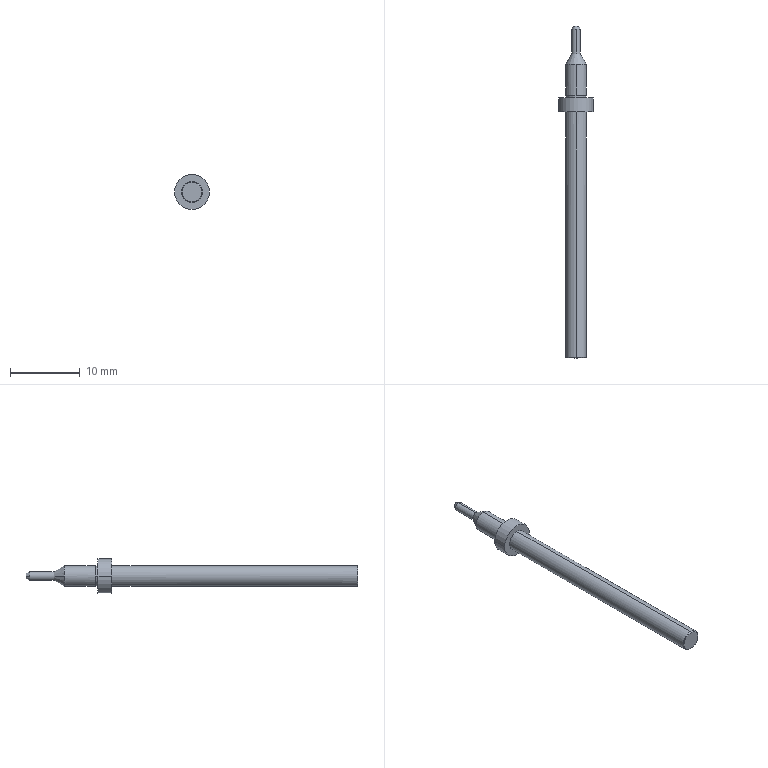Part | NX | 1 solid | 21 faces | box 5 x 47.5 x 5 mm | volume 332.204 mm3 | cylinder 10 | cone 6 | plane 5 | commonest cylinder face diameters 3 x4 1.28 x2 2.8 x2 5 x2
STEP:
#1=CARTESIAN_POINT('',(0.,25.2,-1.5));
#2=VERTEX_POINT('',#1);
#3=CARTESIAN_POINT('',(0.,25.2,1.5));
#4=VERTEX_POINT('',#3);
#5=CARTESIAN_POINT('',(0.,25.2,0.));
#6=DIRECTION('',(0.,-1.,0.));
#7=DIRECTION('',(0.,0.,1.));
#8=AXIS2_PLACEMENT_3D('',#5,#6,#7);
#9=CIRCLE('',#8,1.5);
#10=EDGE_CURVE('',#2,#4,#9,.T.);
#11=ORIENTED_EDGE('',*,*,#10,.T.);
#12=CARTESIAN_POINT('',(0.,-9.9,1.5));
#13=VERTEX_POINT('',#12);
#14=CARTESIAN_POINT('',(0.,39.875,1.5));
#15=DIRECTION('',(0.,-1.,0.));
#16=VECTOR('',#15,1000.);
#17=LINE('',#14,#16);
#18=EDGE_CURVE('',#4,#13,#17,.T.);
#19=ORIENTED_EDGE('',*,*,#18,.T.);
#20=CARTESIAN_POINT('',(1.5,-9.9,0.));
#21=VERTEX_POINT('',#20);
#22=CARTESIAN_POINT('',(0.,-9.9,0.));
#23=DIRECTION('',(0.,1.,0.));
#24=DIRECTION('',(1.,0.,0.));
#25=AXIS2_PLACEMENT_3D('',#22,#23,#24);
#26=CIRCLE('',#25,1.5);
#27=EDGE_CURVE('',#13,#21,#26,.T.);
#28=ORIENTED_EDGE('',*,*,#27,.T.);
#29=CARTESIAN_POINT('',(0.,-9.9,-1.5));
#30=VERTEX_POINT('',#29);
#31=CARTESIAN_POINT('',(0.,-9.9,0.));
#32=DIRECTION('',(0.,1.,0.));
#33=DIRECTION('',(1.,0.,0.));
#34=AXIS2_PLACEMENT_3D('',#31,#32,#33);
#35=CIRCLE('',#34,1.5);
#36=EDGE_CURVE('',#21,#30,#35,.T.);
#37=ORIENTED_EDGE('',*,*,#36,.T.);
#38=CARTESIAN_POINT('',(0.,39.875,-1.5));
#39=DIRECTION('',(0.,-1.,0.));
#40=VECTOR('',#39,1000.);
#41=LINE('',#38,#40);
#42=EDGE_CURVE('',#2,#30,#41,.T.);
#43=ORIENTED_EDGE('',*,*,#42,.F.);
#44=EDGE_LOOP('',(#11,#19,#28,#37,#43));
#45=FACE_BOUND('',#44,.T.);
#46=CARTESIAN_POINT('',(0.,39.875,0.));
#47=DIRECTION('',(0.,-1.,0.));
#48=DIRECTION('',(0.,0.,1.));
#49=AXIS2_PLACEMENT_3D('',#46,#47,#48);
#50=CYLINDRICAL_SURFACE('',#49,1.5);
#51=ADVANCED_FACE('',(#45),#50,.T.);
#52=CARTESIAN_POINT('',(-2.5,25.2,0.));
#53=VERTEX_POINT('',#52);
#54=CARTESIAN_POINT('',(2.5,25.2,0.));
#55=VERTEX_POINT('',#54);
#56=CARTESIAN_POINT('',(0.,25.2,0.));
#57=DIRECTION('',(0.,1.,0.));
#58=DIRECTION('',(1.,0.,0.));
#59=AXIS2_PLACEMENT_3D('',#56,#57,#58);
#60=CIRCLE('',#59,2.5);
#61=EDGE_CURVE('',#53,#55,#60,.T.);
#62=ORIENTED_EDGE('',*,*,#61,.F.);
#63=CARTESIAN_POINT('',(0.,25.2,0.));
#64=DIRECTION('',(0.,1.,0.));
#65=DIRECTION('',(1.,0.,0.));
#66=AXIS2_PLACEMENT_3D('',#63,#64,#65);
#67=CIRCLE('',#66,2.5);
#68=EDGE_CURVE('',#55,#53,#67,.T.);
#69=ORIENTED_EDGE('',*,*,#68,.F.);
#70=EDGE_LOOP('',(#62,#69));
#71=FACE_BOUND('',#70,.T.);
#72=ORIENTED_EDGE('',*,*,#10,.F.);
#73=CARTESIAN_POINT('',(0.,25.2,0.));
#74=DIRECTION('',(0.,-1.,0.));
#75=DIRECTION('',(0.,0.,1.));
#76=AXIS2_PLACEMENT_3D('',#73,#74,#75);
#77=CIRCLE('',#76,1.5);
#78=EDGE_CURVE('',#4,#2,#77,.T.);
#79=ORIENTED_EDGE('',*,*,#78,.F.);
#80=EDGE_LOOP('',(#72,#79));
#81=FACE_BOUND('',#80,.T.);
#82=CARTESIAN_POINT('',(0.,25.2,0.));
#83=DIRECTION('',(0.,-1.,0.));
#84=DIRECTION('',(0.,0.,-1.));
#85=AXIS2_PLACEMENT_3D('',#82,#83,#84);
#86=PLANE('',#85);
#87=ADVANCED_FACE('',(#71,#81),#86,.T.);
#88=CARTESIAN_POINT('',(2.5,27.2,0.));
#89=VERTEX_POINT('',#88);
#90=CARTESIAN_POINT('',(-2.5,27.2,0.));
#91=VERTEX_POINT('',#90);
#92=CARTESIAN_POINT('',(0.,27.2,0.));
#93=DIRECTION('',(0.,-1.,0.));
#94=DIRECTION('',(-1.,0.,0.));
#95=AXIS2_PLACEMENT_3D('',#92,#93,#94);
#96=CIRCLE('',#95,2.5);
#97=EDGE_CURVE('',#89,#91,#96,.T.);
#98=ORIENTED_EDGE('',*,*,#97,.T.);
#99=CARTESIAN_POINT('',(-2.5,27.2,0.));
#100=DIRECTION('',(0.,-1.,0.));
#101=VECTOR('',#100,1000.);
#102=LINE('',#99,#101);
#103=EDGE_CURVE('',#91,#53,#102,.T.);
#104=ORIENTED_EDGE('',*,*,#103,.T.);
#105=ORIENTED_EDGE('',*,*,#61,.T.);
#106=CARTESIAN_POINT('',(2.5,27.2,0.));
#107=DIRECTION('',(0.,-1.,0.));
#108=VECTOR('',#107,1000.);
#109=LINE('',#106,#108);
#110=EDGE_CURVE('',#89,#55,#109,.T.);
#111=ORIENTED_EDGE('',*,*,#110,.F.);
#112=EDGE_LOOP('',(#98,#104,#105,#111));
#113=FACE_BOUND('',#112,.T.);
#114=CARTESIAN_POINT('',(0.,27.2,0.));
#115=DIRECTION('',(0.,-1.,0.));
#116=DIRECTION('',(1.,0.,0.));
#117=AXIS2_PLACEMENT_3D('',#114,#115,#116);
#118=CYLINDRICAL_SURFACE('',#117,2.5);
#119=ADVANCED_FACE('',(#113),#118,.T.);
#120=CARTESIAN_POINT('',(0.,27.6,1.5));
#121=VERTEX_POINT('',#120);
#122=CARTESIAN_POINT('',(0.,27.6,-1.5));
#123=VERTEX_POINT('',#122);
#124=CARTESIAN_POINT('',(0.,27.6,0.));
#125=DIRECTION('',(0.,-1.,0.));
#126=DIRECTION('',(0.,0.,1.));
#127=AXIS2_PLACEMENT_3D('',#124,#125,#126);
#128=CIRCLE('',#127,1.5);
#129=EDGE_CURVE('',#121,#123,#128,.T.);
#130=ORIENTED_EDGE('',*,*,#129,.T.);
#131=CARTESIAN_POINT('',(0.,27.6,0.));
#132=DIRECTION('',(0.,-1.,0.));
#133=DIRECTION('',(0.,0.,1.));
#134=AXIS2_PLACEMENT_3D('',#131,#132,#133);
#135=CIRCLE('',#134,1.5);
#136=EDGE_CURVE('',#123,#121,#135,.T.);
#137=ORIENTED_EDGE('',*,*,#136,.T.);
#138=EDGE_LOOP('',(#130,#137));
#139=FACE_BOUND('',#138,.T.);
#140=CARTESIAN_POINT('',(1.4,27.6,0.));
#141=VERTEX_POINT('',#140);
#142=CARTESIAN_POINT('',(-1.4,27.6,0.));
#143=VERTEX_POINT('',#142);
#144=CARTESIAN_POINT('',(0.,27.6,0.));
#145=DIRECTION('',(0.,1.,0.));
#146=DIRECTION('',(1.,0.,0.));
#147=AXIS2_PLACEMENT_3D('',#144,#145,#146);
#148=CIRCLE('',#147,1.4);
#149=EDGE_CURVE('',#141,#143,#148,.T.);
#150=ORIENTED_EDGE('',*,*,#149,.T.);
#151=CARTESIAN_POINT('',(0.,27.6,0.));
#152=DIRECTION('',(0.,1.,0.));
#153=DIRECTION('',(1.,0.,0.));
#154=AXIS2_PLACEMENT_3D('',#151,#152,#153);
#155=CIRCLE('',#154,1.4);
#156=EDGE_CURVE('',#143,#141,#155,.T.);
#157=ORIENTED_EDGE('',*,*,#156,.T.);
#158=EDGE_LOOP('',(#150,#157));
#159=FACE_BOUND('',#158,.T.);
#160=CARTESIAN_POINT('',(0.,27.6,0.));
#161=DIRECTION('',(0.,1.,0.));
#162=DIRECTION('',(1.,0.,0.));
#163=AXIS2_PLACEMENT_3D('',#160,#161,#162);
#164=PLANE('',#163);
#165=ADVANCED_FACE('',(#139,#159),#164,.F.);
#166=CARTESIAN_POINT('',(-1.4,-10.,0.));
#167=VERTEX_POINT('',#166);
#168=CARTESIAN_POINT('',(1.4,-10.,0.));
#169=VERTEX_POINT('',#168);
#170=CARTESIAN_POINT('',(0.,-10.,0.));
#171=DIRECTION('',(0.,1.,0.));
#172=DIRECTION('',(1.,0.,0.));
#173=AXIS2_PLACEMENT_3D('',#170,#171,#172);
#174=CIRCLE('',#173,1.4);
#175=EDGE_CURVE('',#167,#169,#174,.T.);
#176=ORIENTED_EDGE('',*,*,#175,.F.);
#177=CARTESIAN_POINT('',(0.,-10.,0.));
#178=DIRECTION('',(0.,1.,0.));
#179=DIRECTION('',(1.,0.,0.));
#180=AXIS2_PLACEMENT_3D('',#177,#178,#179);
#181=CIRCLE('',#180,1.4);
#182=EDGE_CURVE('',#169,#167,#181,.T.);
#183=ORIENTED_EDGE('',*,*,#182,.F.);
#184=EDGE_LOOP('',(#176,#183));
#185=FACE_BOUND('',#184,.T.);
#186=CARTESIAN_POINT('',(0.,-10.,0.));
#187=DIRECTION('',(0.,-1.,0.));
#188=DIRECTION('',(0.,0.,-1.));
#189=AXIS2_PLACEMENT_3D('',#186,#187,#188);
#190=PLANE('',#189);
#191=ADVANCED_FACE('',(#185),#190,.T.);
#192=CARTESIAN_POINT('',(1.4,27.2,0.));
#193=VERTEX_POINT('',#192);
#194=CARTESIAN_POINT('',(-1.4,27.2,0.));
#195=VERTEX_POINT('',#194);
#196=CARTESIAN_POINT('',(0.,27.2,0.));
#197=DIRECTION('',(0.,1.,0.));
#198=DIRECTION('',(1.,0.,0.));
#199=AXIS2_PLACEMENT_3D('',#196,#197,#198);
#200=CIRCLE('',#199,1.4);
#201=EDGE_CURVE('',#193,#195,#200,.T.);
#202=ORIENTED_EDGE('',*,*,#201,.T.);
#203=CARTESIAN_POINT('',(-1.4,27.195,0.));
#204=DIRECTION('',(0.,1.,0.));
#205=VECTOR('',#204,1000.);
#206=LINE('',#203,#205);
#207=EDGE_CURVE('',#195,#143,#206,.T.);
#208=ORIENTED_EDGE('',*,*,#207,.T.);
#209=ORIENTED_EDGE('',*,*,#149,.F.);
#210=CARTESIAN_POINT('',(1.4,27.195,0.));
#211=DIRECTION('',(0.,1.,0.));
#212=VECTOR('',#211,1000.);
#213=LINE('',#210,#212);
#214=EDGE_CURVE('',#193,#141,#213,.T.);
#215=ORIENTED_EDGE('',*,*,#214,.F.);
#216=EDGE_LOOP('',(#202,#208,#209,#215));
#217=FACE_BOUND('',#216,.T.);
#218=CARTESIAN_POINT('',(0.,27.195,0.));
#219=DIRECTION('',(0.,1.,0.));
#220=DIRECTION('',(1.,0.,0.));
#221=AXIS2_PLACEMENT_3D('',#218,#219,#220);
#222=CYLINDRICAL_SURFACE('',#221,1.4);
#223=ADVANCED_FACE('',(#217),#222,.T.);
#224=CARTESIAN_POINT('',(0.4068,37.5,0.));
#225=VERTEX_POINT('',#224);
#226=CARTESIAN_POINT('',(-0.4068,37.5,0.));
#227=VERTEX_POINT('',#226);
#228=CARTESIAN_POINT('',(0.,37.5,0.));
#229=DIRECTION('',(0.,-1.,0.));
#230=DIRECTION('',(-1.,0.,0.));
#231=AXIS2_PLACEMENT_3D('',#228,#229,#230);
#232=CIRCLE('',#231,0.4068);
#233=EDGE_CURVE('',#225,#227,#232,.T.);
#234=ORIENTED_EDGE('',*,*,#233,.F.);
#235=CARTESIAN_POINT('',(0.,37.5,0.));
#236=DIRECTION('',(0.,-1.,0.));
#237=DIRECTION('',(-1.,0.,0.));
#238=AXIS2_PLACEMENT_3D('',#235,#236,#237);
#239=CIRCLE('',#238,0.4068);
#240=EDGE_CURVE('',#227,#225,#239,.T.);
#241=ORIENTED_EDGE('',*,*,#240,.F.);
#242=EDGE_LOOP('',(#234,#241));
#243=FACE_BOUND('',#242,.T.);
#244=CARTESIAN_POINT('',(0.,37.5,0.));
#245=DIRECTION('',(0.,-1.,0.));
#246=DIRECTION('',(0.,0.,-1.));
#247=AXIS2_PLACEMENT_3D('',#244,#245,#246);
#248=PLANE('',#247);
#249=ADVANCED_FACE('',(#243),#248,.F.);
#250=ORIENTED_EDGE('',*,*,#97,.F.);
#251=CARTESIAN_POINT('',(0.,27.2,0.));
#252=DIRECTION('',(0.,-1.,0.));
#253=DIRECTION('',(-1.,0.,0.));
#254=AXIS2_PLACEMENT_3D('',#251,#252,#253);
#255=CIRCLE('',#254,2.5);
#256=EDGE_CURVE('',#91,#89,#255,.T.);
#257=ORIENTED_EDGE('',*,*,#256,.F.);
#258=EDGE_LOOP('',(#250,#257));
#259=FACE_BOUND('',#258,.T.);
#260=ORIENTED_EDGE('',*,*,#201,.F.);
#261=CARTESIAN_POINT('',(0.,27.2,0.));
#262=DIRECTION('',(0.,1.,0.));
#263=DIRECTION('',(1.,0.,0.));
#264=AXIS2_PLACEMENT_3D('',#261,#262,#263);
#265=CIRCLE('',#264,1.4);
#266=EDGE_CURVE('',#195,#193,#265,.T.);
#267=ORIENTED_EDGE('',*,*,#266,.F.);
#268=EDGE_LOOP('',(#260,#267));
#269=FACE_BOUND('',#268,.T.);
#270=CARTESIAN_POINT('',(0.,27.2,0.));
#271=DIRECTION('',(0.,-1.,0.));
#272=DIRECTION('',(0.,0.,-1.));
#273=AXIS2_PLACEMENT_3D('',#270,#271,#272);
#274=PLANE('',#273);
#275=ADVANCED_FACE('',(#259,#269),#274,.F.);
#276=CARTESIAN_POINT('',(-1.5,32.,0.));
#277=VERTEX_POINT('',#276);
#278=CARTESIAN_POINT('',(0.,32.,-1.5));
#279=VERTEX_POINT('',#278);
#280=CARTESIAN_POINT('',(0.,32.,0.));
#281=DIRECTION('',(0.,-1.,0.));
#282=DIRECTION('',(-1.,0.,0.));
#283=AXIS2_PLACEMENT_3D('',#280,#281,#282);
#284=CIRCLE('',#283,1.5);
#285=EDGE_CURVE('',#277,#279,#284,.T.);
#286=ORIENTED_EDGE('',*,*,#285,.T.);
#287=CARTESIAN_POINT('',(0.,39.875,-1.5));
#288=DIRECTION('',(0.,-1.,0.));
#289=VECTOR('',#288,1000.);
#290=LINE('',#287,#289);
#291=EDGE_CURVE('',#279,#123,#290,.T.);
#292=ORIENTED_EDGE('',*,*,#291,.T.);
#293=ORIENTED_EDGE('',*,*,#129,.F.);
#294=CARTESIAN_POINT('',(0.,32.,1.5));
#295=VERTEX_POINT('',#294);
#296=CARTESIAN_POINT('',(0.,39.875,1.5));
#297=DIRECTION('',(0.,-1.,0.));
#298=VECTOR('',#297,1000.);
#299=LINE('',#296,#298);
#300=EDGE_CURVE('',#295,#121,#299,.T.);
#301=ORIENTED_EDGE('',*,*,#300,.F.);
#302=CARTESIAN_POINT('',(0.,32.,0.));
#303=DIRECTION('',(0.,-1.,0.));
#304=DIRECTION('',(-1.,0.,0.));
#305=AXIS2_PLACEMENT_3D('',#302,#303,#304);
#306=CIRCLE('',#305,1.5);
#307=EDGE_CURVE('',#295,#277,#306,.T.);
#308=ORIENTED_EDGE('',*,*,#307,.T.);
#309=EDGE_LOOP('',(#286,#292,#293,#301,#308));
#310=FACE_BOUND('',#309,.T.);
#311=CARTESIAN_POINT('',(0.,39.875,0.));
#312=DIRECTION('',(0.,-1.,0.));
#313=DIRECTION('',(0.,0.,1.));
#314=AXIS2_PLACEMENT_3D('',#311,#312,#313);
#315=CYLINDRICAL_SURFACE('',#314,1.5);
#316=ADVANCED_FACE('',(#310),#315,.T.);
#317=CARTESIAN_POINT('',(0.,37.,0.64));
#318=VERTEX_POINT('',#317);
#319=CARTESIAN_POINT('',(-0.64,37.,0.));
#320=VERTEX_POINT('',#319);
#321=CARTESIAN_POINT('',(0.,37.,0.));
#322=DIRECTION('',(0.,-1.,0.));
#323=DIRECTION('',(-1.,0.,0.));
#324=AXIS2_PLACEMENT_3D('',#321,#322,#323);
#325=CIRCLE('',#324,0.64);
#326=EDGE_CURVE('',#318,#320,#325,.T.);
#327=ORIENTED_EDGE('',*,*,#326,.T.);
#328=CARTESIAN_POINT('',(0.,37.,-0.64));
#329=VERTEX_POINT('',#328);
#330=CARTESIAN_POINT('',(0.,37.,0.));
#331=DIRECTION('',(0.,-1.,0.));
#332=DIRECTION('',(-1.,0.,0.));
#333=AXIS2_PLACEMENT_3D('',#330,#331,#332);
#334=CIRCLE('',#333,0.64);
#335=EDGE_CURVE('',#320,#329,#334,.T.);
#336=ORIENTED_EDGE('',*,*,#335,.T.);
#337=CARTESIAN_POINT('',(0.,33.49,-0.64));
#338=VERTEX_POINT('',#337);
#339=CARTESIAN_POINT('',(0.,39.875,-0.64));
#340=DIRECTION('',(0.,-1.,0.));
#341=VECTOR('',#340,1000.);
#342=LINE('',#339,#341);
#343=EDGE_CURVE('',#338,#329,#342,.F.);
#344=ORIENTED_EDGE('',*,*,#343,.F.);
#345=CARTESIAN_POINT('',(-0.64,33.49,0.));
#346=VERTEX_POINT('',#345);
#347=CARTESIAN_POINT('',(0.,33.49,0.));
#348=DIRECTION('',(0.,-1.,0.));
#349=DIRECTION('',(-1.,0.,0.));
#350=AXIS2_PLACEMENT_3D('',#347,#348,#349);
#351=CIRCLE('',#350,0.64);
#352=EDGE_CURVE('',#346,#338,#351,.T.);
#353=ORIENTED_EDGE('',*,*,#352,.F.);
#354=CARTESIAN_POINT('',(0.,33.49,0.64));
#355=VERTEX_POINT('',#354);
#356=CARTESIAN_POINT('',(0.,33.49,0.));
#357=DIRECTION('',(0.,-1.,0.));
#358=DIRECTION('',(-1.,0.,0.));
#359=AXIS2_PLACEMENT_3D('',#356,#357,#358);
#360=CIRCLE('',#359,0.64);
#361=EDGE_CURVE('',#355,#346,#360,.T.);
#362=ORIENTED_EDGE('',*,*,#361,.F.);
#363=CARTESIAN_POINT('',(0.,39.875,0.64));
#364=DIRECTION('',(0.,-1.,0.));
#365=VECTOR('',#364,1000.);
#366=LINE('',#363,#365);
#367=EDGE_CURVE('',#355,#318,#366,.F.);
#368=ORIENTED_EDGE('',*,*,#367,.T.);
#369=EDGE_LOOP('',(#327,#336,#344,#353,#362,#368));
#370=FACE_BOUND('',#369,.T.);
#371=CARTESIAN_POINT('',(0.,39.875,0.));
#372=DIRECTION('',(0.,-1.,0.));
#373=DIRECTION('',(0.,0.,1.));
#374=AXIS2_PLACEMENT_3D('',#371,#372,#373);
#375=CYLINDRICAL_SURFACE('',#374,0.64);
#376=ADVANCED_FACE('',(#370),#375,.T.);
#377=ORIENTED_EDGE('',*,*,#285,.F.);
#378=CARTESIAN_POINT('',(-1.07,32.745,0.));
#379=DIRECTION('',(-0.5,-0.866,0.));
#380=VECTOR('',#379,1000.);
#381=LINE('',#378,#380);
#382=EDGE_CURVE('',#277,#346,#381,.F.);
#383=ORIENTED_EDGE('',*,*,#382,.T.);
#384=ORIENTED_EDGE('',*,*,#352,.T.);
#385=CARTESIAN_POINT('',(0.64,33.49,0.));
#386=VERTEX_POINT('',#385);
#387=CARTESIAN_POINT('',(0.,33.49,0.));
#388=DIRECTION('',(0.,-1.,0.));
#389=DIRECTION('',(-1.,0.,0.));
#390=AXIS2_PLACEMENT_3D('',#387,#388,#389);
#391=CIRCLE('',#390,0.64);
#392=EDGE_CURVE('',#338,#386,#391,.T.);
#393=ORIENTED_EDGE('',*,*,#392,.T.);
#394=CARTESIAN_POINT('',(1.5,32.,0.));
#395=VERTEX_POINT('',#394);
#396=CARTESIAN_POINT('',(1.07,32.745,0.));
#397=DIRECTION('',(0.5,-0.866,0.));
#398=VECTOR('',#397,1000.);
#399=LINE('',#396,#398);
#400=EDGE_CURVE('',#395,#386,#399,.F.);
#401=ORIENTED_EDGE('',*,*,#400,.F.);
#402=CARTESIAN_POINT('',(0.,32.,0.));
#403=DIRECTION('',(0.,-1.,0.));
#404=DIRECTION('',(-1.,0.,0.));
#405=AXIS2_PLACEMENT_3D('',#402,#403,#404);
#406=CIRCLE('',#405,1.5);
#407=EDGE_CURVE('',#279,#395,#406,.T.);
#408=ORIENTED_EDGE('',*,*,#407,.F.);
#409=EDGE_LOOP('',(#377,#383,#384,#393,#401,#408));
#410=FACE_BOUND('',#409,.T.);
#411=CARTESIAN_POINT('',(0.,32.745,0.));
#412=DIRECTION('',(0.,-1.,0.));
#413=DIRECTION('',(-1.,0.,0.));
#414=AXIS2_PLACEMENT_3D('',#411,#412,#413);
#415=CONICAL_SURFACE('',#414,1.07,0.5236);
#416=ADVANCED_FACE('',(#410),#415,.T.);
#417=ORIENTED_EDGE('',*,*,#326,.F.);
#418=CARTESIAN_POINT('',(0.64,37.,0.));
#419=VERTEX_POINT('',#418);
#420=CARTESIAN_POINT('',(0.,37.,0.));
#421=DIRECTION('',(0.,-1.,0.));
#422=DIRECTION('',(-1.,0.,0.));
#423=AXIS2_PLACEMENT_3D('',#420,#421,#422);
#424=CIRCLE('',#423,0.64);
#425=EDGE_CURVE('',#419,#318,#424,.T.);
#426=ORIENTED_EDGE('',*,*,#425,.F.);
#427=CARTESIAN_POINT('',(0.64,37.,0.));
#428=DIRECTION('',(0.4226,-0.9063,0.));
#429=VECTOR('',#428,1000.);
#430=LINE('',#427,#429);
#431=EDGE_CURVE('',#419,#225,#430,.F.);
#432=ORIENTED_EDGE('',*,*,#431,.T.);
#433=ORIENTED_EDGE('',*,*,#233,.T.);
#434=CARTESIAN_POINT('',(-0.64,37.,0.));
#435=DIRECTION('',(-0.4226,-0.9063,0.));
#436=VECTOR('',#435,1000.);
#437=LINE('',#434,#436);
#438=EDGE_CURVE('',#320,#227,#437,.F.);
#439=ORIENTED_EDGE('',*,*,#438,.F.);
#440=EDGE_LOOP('',(#417,#426,#432,#433,#439));
#441=FACE_BOUND('',#440,.T.);
#442=CARTESIAN_POINT('',(0.,37.,0.));
#443=DIRECTION('',(0.,-1.,0.));
#444=DIRECTION('',(-1.,0.,0.));
#445=AXIS2_PLACEMENT_3D('',#442,#443,#444);
#446=CONICAL_SURFACE('',#445,0.64,0.4363);
#447=ADVANCED_FACE('',(#441),#446,.T.);
#448=ORIENTED_EDGE('',*,*,#175,.T.);
#449=CARTESIAN_POINT('',(1.5,-9.9,0.));
#450=DIRECTION('',(0.7071,0.7071,0.));
#451=VECTOR('',#450,1000.);
#452=LINE('',#449,#451);
#453=EDGE_CURVE('',#169,#21,#452,.T.);
#454=ORIENTED_EDGE('',*,*,#453,.T.);
#455=ORIENTED_EDGE('',*,*,#27,.F.);
#456=CARTESIAN_POINT('',(-1.5,-9.9,0.));
#457=VERTEX_POINT('',#456);
#458=CARTESIAN_POINT('',(0.,-9.9,0.));
#459=DIRECTION('',(0.,1.,0.));
#460=DIRECTION('',(1.,0.,0.));
#461=AXIS2_PLACEMENT_3D('',#458,#459,#460);
#462=CIRCLE('',#461,1.5);
#463=EDGE_CURVE('',#457,#13,#462,.T.);
#464=ORIENTED_EDGE('',*,*,#463,.F.);
#465=CARTESIAN_POINT('',(-1.5,-9.9,0.));
#466=DIRECTION('',(-0.7071,0.7071,0.));
#467=VECTOR('',#466,1000.);
#468=LINE('',#465,#467);
#469=EDGE_CURVE('',#167,#457,#468,.T.);
#470=ORIENTED_EDGE('',*,*,#469,.F.);
#471=EDGE_LOOP('',(#448,#454,#455,#464,#470));
#472=FACE_BOUND('',#471,.T.);
#473=CARTESIAN_POINT('',(0.,-9.9,0.));
#474=DIRECTION('',(0.,1.,0.));
#475=DIRECTION('',(1.,0.,0.));
#476=AXIS2_PLACEMENT_3D('',#473,#474,#475);
#477=CONICAL_SURFACE('',#476,1.5,0.7854);
#478=ADVANCED_FACE('',(#472),#477,.T.);
#479=ORIENTED_EDGE('',*,*,#382,.F.);
#480=ORIENTED_EDGE('',*,*,#307,.F.);
#481=CARTESIAN_POINT('',(0.,32.,0.));
#482=DIRECTION('',(0.,-1.,0.));
#483=DIRECTION('',(-1.,0.,0.));
#484=AXIS2_PLACEMENT_3D('',#481,#482,#483);
#485=CIRCLE('',#484,1.5);
#486=EDGE_CURVE('',#395,#295,#485,.T.);
#487=ORIENTED_EDGE('',*,*,#486,.F.);
#488=ORIENTED_EDGE('',*,*,#400,.T.);
#489=CARTESIAN_POINT('',(0.,33.49,0.));
#490=DIRECTION('',(0.,-1.,0.));
#491=DIRECTION('',(-1.,0.,0.));
#492=AXIS2_PLACEMENT_3D('',#489,#490,#491);
#493=CIRCLE('',#492,0.64);
#494=EDGE_CURVE('',#386,#355,#493,.T.);
#495=ORIENTED_EDGE('',*,*,#494,.T.);
#496=ORIENTED_EDGE('',*,*,#361,.T.);
#497=EDGE_LOOP('',(#479,#480,#487,#488,#495,#496));
#498=FACE_BOUND('',#497,.T.);
#499=CARTESIAN_POINT('',(0.,32.745,0.));
#500=DIRECTION('',(0.,-1.,0.));
#501=DIRECTION('',(-1.,0.,0.));
#502=AXIS2_PLACEMENT_3D('',#499,#500,#501);
#503=CONICAL_SURFACE('',#502,1.07,0.5236);
#504=ADVANCED_FACE('',(#498),#503,.T.);
#505=ORIENTED_EDGE('',*,*,#214,.T.);
#506=ORIENTED_EDGE('',*,*,#156,.F.);
#507=ORIENTED_EDGE('',*,*,#207,.F.);
#508=ORIENTED_EDGE('',*,*,#266,.T.);
#509=EDGE_LOOP('',(#505,#506,#507,#508));
#510=FACE_BOUND('',#509,.T.);
#511=CARTESIAN_POINT('',(0.,27.195,0.));
#512=DIRECTION('',(0.,1.,0.));
#513=DIRECTION('',(1.,0.,0.));
#514=AXIS2_PLACEMENT_3D('',#511,#512,#513);
#515=CYLINDRICAL_SURFACE('',#514,1.4);
#516=ADVANCED_FACE('',(#510),#515,.T.);
#517=ORIENTED_EDGE('',*,*,#453,.F.);
#518=ORIENTED_EDGE('',*,*,#182,.T.);
#519=ORIENTED_EDGE('',*,*,#469,.T.);
#520=CARTESIAN_POINT('',(0.,-9.9,0.));
#521=DIRECTION('',(0.,1.,0.));
#522=DIRECTION('',(1.,0.,0.));
#523=AXIS2_PLACEMENT_3D('',#520,#521,#522);
#524=CIRCLE('',#523,1.5);
#525=EDGE_CURVE('',#30,#457,#524,.T.);
#526=ORIENTED_EDGE('',*,*,#525,.F.);
#527=ORIENTED_EDGE('',*,*,#36,.F.);
#528=EDGE_LOOP('',(#517,#518,#519,#526,#527));
#529=FACE_BOUND('',#528,.T.);
#530=CARTESIAN_POINT('',(0.,-9.9,0.));
#531=DIRECTION('',(0.,1.,0.));
#532=DIRECTION('',(1.,0.,0.));
#533=AXIS2_PLACEMENT_3D('',#530,#531,#532);
#534=CONICAL_SURFACE('',#533,1.5,0.7854);
#535=ADVANCED_FACE('',(#529),#534,.T.);
#536=ORIENTED_EDGE('',*,*,#392,.F.);
#537=ORIENTED_EDGE('',*,*,#343,.T.);
#538=CARTESIAN_POINT('',(0.,37.,0.));
#539=DIRECTION('',(0.,-1.,0.));
#540=DIRECTION('',(-1.,0.,0.));
#541=AXIS2_PLACEMENT_3D('',#538,#539,#540);
#542=CIRCLE('',#541,0.64);
#543=EDGE_CURVE('',#329,#419,#542,.T.);
#544=ORIENTED_EDGE('',*,*,#543,.T.);
#545=ORIENTED_EDGE('',*,*,#425,.T.);
#546=ORIENTED_EDGE('',*,*,#367,.F.);
#547=ORIENTED_EDGE('',*,*,#494,.F.);
#548=EDGE_LOOP('',(#536,#537,#544,#545,#546,#547));
#549=FACE_BOUND('',#548,.T.);
#550=CARTESIAN_POINT('',(0.,39.875,0.));
#551=DIRECTION('',(0.,-1.,0.));
#552=DIRECTION('',(0.,0.,1.));
#553=AXIS2_PLACEMENT_3D('',#550,#551,#552);
#554=CYLINDRICAL_SURFACE('',#553,0.64);
#555=ADVANCED_FACE('',(#549),#554,.T.);
#556=ORIENTED_EDGE('',*,*,#110,.T.);
#557=ORIENTED_EDGE('',*,*,#68,.T.);
#558=ORIENTED_EDGE('',*,*,#103,.F.);
#559=ORIENTED_EDGE('',*,*,#256,.T.);
#560=EDGE_LOOP('',(#556,#557,#558,#559));
#561=FACE_BOUND('',#560,.T.);
#562=CARTESIAN_POINT('',(0.,27.2,0.));
#563=DIRECTION('',(0.,-1.,0.));
#564=DIRECTION('',(1.,0.,0.));
#565=AXIS2_PLACEMENT_3D('',#562,#563,#564);
#566=CYLINDRICAL_SURFACE('',#565,2.5);
#567=ADVANCED_FACE('',(#561),#566,.T.);
#568=ORIENTED_EDGE('',*,*,#438,.T.);
#569=ORIENTED_EDGE('',*,*,#240,.T.);
#570=ORIENTED_EDGE('',*,*,#431,.F.);
#571=ORIENTED_EDGE('',*,*,#543,.F.);
#572=ORIENTED_EDGE('',*,*,#335,.F.);
#573=EDGE_LOOP('',(#568,#569,#570,#571,#572));
#574=FACE_BOUND('',#573,.T.);
#575=CARTESIAN_POINT('',(0.,37.,0.));
#576=DIRECTION('',(0.,-1.,0.));
#577=DIRECTION('',(-1.,0.,0.));
#578=AXIS2_PLACEMENT_3D('',#575,#576,#577);
#579=CONICAL_SURFACE('',#578,0.64,0.4363);
#580=ADVANCED_FACE('',(#574),#579,.T.);
#581=ORIENTED_EDGE('',*,*,#300,.T.);
#582=ORIENTED_EDGE('',*,*,#136,.F.);
#583=ORIENTED_EDGE('',*,*,#291,.F.);
#584=ORIENTED_EDGE('',*,*,#407,.T.);
#585=ORIENTED_EDGE('',*,*,#486,.T.);
#586=EDGE_LOOP('',(#581,#582,#583,#584,#585));
#587=FACE_BOUND('',#586,.T.);
#588=CARTESIAN_POINT('',(0.,39.875,0.));
#589=DIRECTION('',(0.,-1.,0.));
#590=DIRECTION('',(0.,0.,1.));
#591=AXIS2_PLACEMENT_3D('',#588,#589,#590);
#592=CYLINDRICAL_SURFACE('',#591,1.5);
#593=ADVANCED_FACE('',(#587),#592,.T.);
#594=ORIENTED_EDGE('',*,*,#463,.T.);
#595=ORIENTED_EDGE('',*,*,#18,.F.);
#596=ORIENTED_EDGE('',*,*,#78,.T.);
#597=ORIENTED_EDGE('',*,*,#42,.T.);
#598=ORIENTED_EDGE('',*,*,#525,.T.);
#599=EDGE_LOOP('',(#594,#595,#596,#597,#598));
#600=FACE_BOUND('',#599,.T.);
#601=CARTESIAN_POINT('',(0.,39.875,0.));
#602=DIRECTION('',(0.,-1.,0.));
#603=DIRECTION('',(0.,0.,1.));
#604=AXIS2_PLACEMENT_3D('',#601,#602,#603);
#605=CYLINDRICAL_SURFACE('',#604,1.5);
#606=ADVANCED_FACE('',(#600),#605,.T.);
#607=CLOSED_SHELL('',(#51,#87,#119,#165,#191,#223,#249,#275,#316,#376,#416,#447,#478,#504,#516,#535,#555,#567,#580,#593,#606));
#608=MANIFOLD_SOLID_BREP('',#607);
#609=(LENGTH_UNIT()NAMED_UNIT(*)SI_UNIT(.MILLI.,.METRE.));
#610=UNCERTAINTY_MEASURE_WITH_UNIT(LENGTH_MEASURE(0.00001),#609,'','');
#611=(NAMED_UNIT(*)PLANE_ANGLE_UNIT()SI_UNIT($,.RADIAN.));
#612=(NAMED_UNIT(*)SI_UNIT($,.STERADIAN.)SOLID_ANGLE_UNIT());
#613=(GEOMETRIC_REPRESENTATION_CONTEXT(3)GLOBAL_UNCERTAINTY_ASSIGNED_CONTEXT((#610))GLOBAL_UNIT_ASSIGNED_CONTEXT((#609,#611,#612))REPRESENTATION_CONTEXT('',''));
#614=ADVANCED_BREP_SHAPE_REPRESENTATION('',(#608),#613);